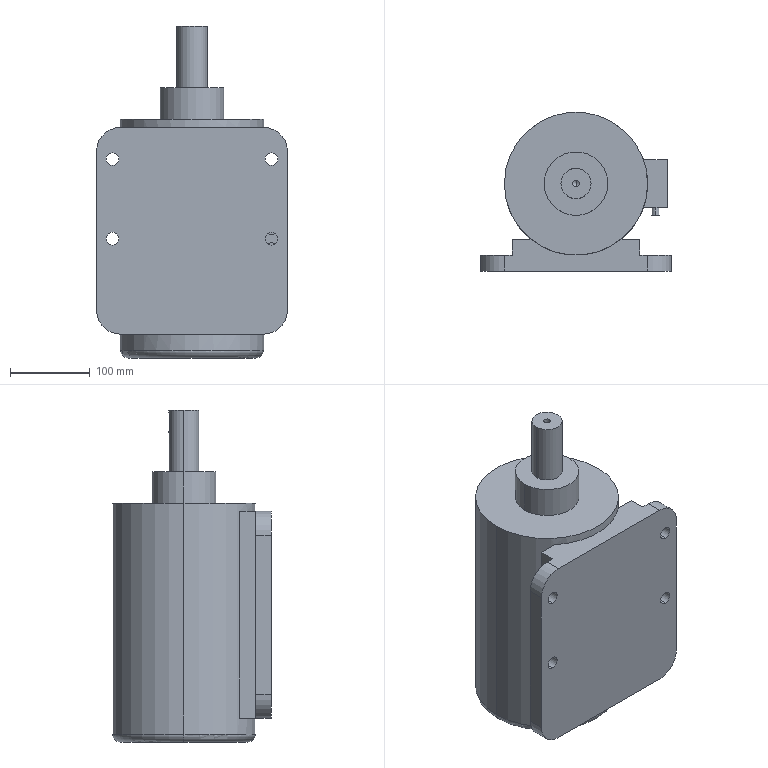Part | SolidWorks | 1 solid | 59 faces | box 240 x 200 x 417.5 mm | volume 9686675 mm3 | cylinder 29 | plane 26 | torus 2 | cone 2 | commonest cylinder face diameters 16 x8 10 x6 60 x4 12 x3 8.5 x2 38 x2